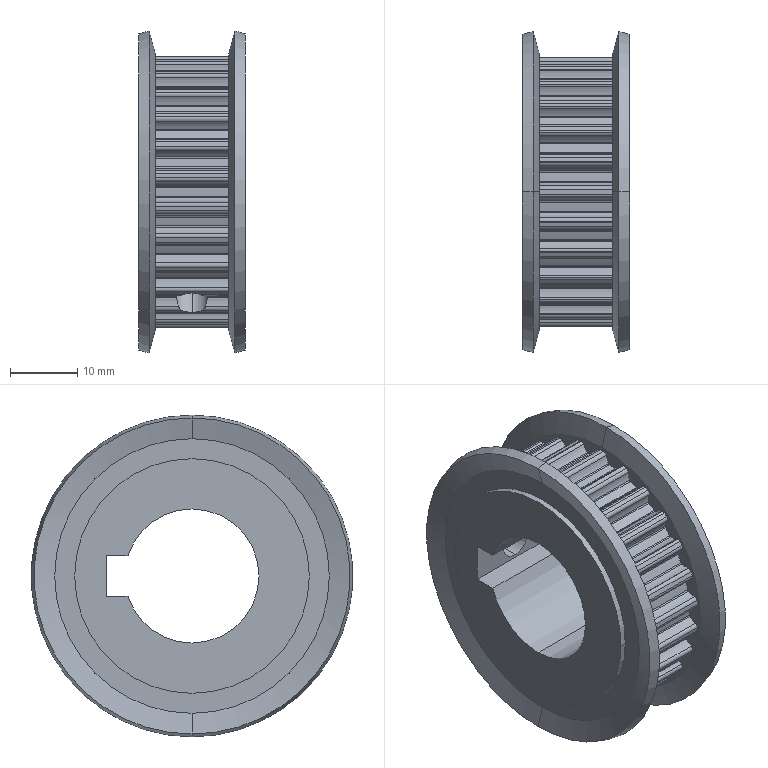Part | SolidWorks | features ICE 3, Fillet 2, HoleWzd 2, BaseBody 1, RevCut 1 | 1 solid | 279 faces | box 16 x 48 x 48 mm | volume 14625 mm3 | cylinder 256 | cone 12 | plane 11 | commonest cylinder face diameters 0.5 x66 1.1 x66 6.55 x58 36.88 x28 40.42 x27 5 x4